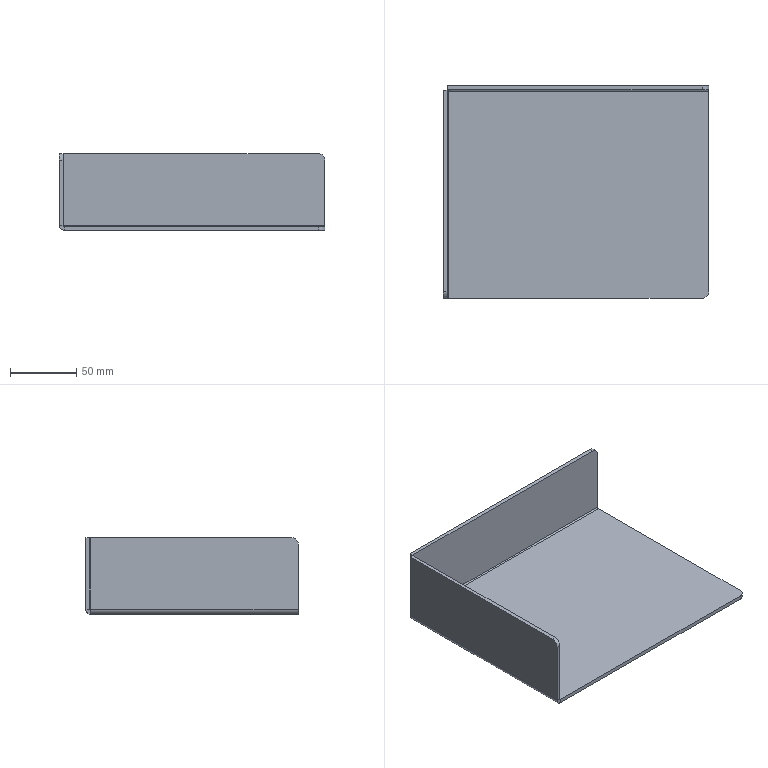Part | SolidWorks | features EdgeFlange 1, Fillet 1, FlatPattern 1, SMBaseFlange 1, SheetMetal 1 | 1 solid | 25 faces | box 200 x 160 x 58 mm | volume 153068 mm3 | plane 16 | cylinder 7 | spline 2 | commonest cylinder face diameters 10 x3 2 x2 8 x2
STEP:
#1=CARTESIAN_POINT('',(0.,5.,-3.));
#2=VERTEX_POINT('',#1);
#3=CARTESIAN_POINT('',(0.,156.,-3.));
#4=VERTEX_POINT('',#3);
#5=CARTESIAN_POINT('',(0.,0.,-3.));
#6=DIRECTION('',(0.,1.,0.));
#7=VECTOR('',#6,1000.);
#8=LINE('',#5,#7);
#9=EDGE_CURVE('',#2,#4,#8,.T.);
#10=ORIENTED_EDGE('',*,*,#9,.F.);
#11=CARTESIAN_POINT('',(-5.,0.,-3.));
#12=VERTEX_POINT('',#11);
#13=CARTESIAN_POINT('',(-5.,5.,-3.));
#14=DIRECTION('',(0.,0.,-1.));
#15=DIRECTION('',(1.,0.,0.));
#16=AXIS2_PLACEMENT_3D('',#13,#14,#15);
#17=CIRCLE('',#16,5.);
#18=EDGE_CURVE('',#2,#12,#17,.T.);
#19=ORIENTED_EDGE('',*,*,#18,.T.);
#20=CARTESIAN_POINT('',(-196.,0.,-3.));
#21=VERTEX_POINT('',#20);
#22=CARTESIAN_POINT('',(0.,0.,-3.));
#23=DIRECTION('',(1.,0.,0.));
#24=VECTOR('',#23,1000.);
#25=LINE('',#22,#24);
#26=EDGE_CURVE('',#21,#12,#25,.T.);
#27=ORIENTED_EDGE('',*,*,#26,.F.);
#28=CARTESIAN_POINT('',(-196.,156.,-3.));
#29=VERTEX_POINT('',#28);
#30=CARTESIAN_POINT('',(-196.,0.,-3.));
#31=DIRECTION('',(0.,1.,0.));
#32=VECTOR('',#31,1000.);
#33=LINE('',#30,#32);
#34=EDGE_CURVE('',#21,#29,#33,.T.);
#35=ORIENTED_EDGE('',*,*,#34,.T.);
#36=CARTESIAN_POINT('',(-196.646,156.,-3.));
#37=DIRECTION('',(1.,0.,0.));
#38=VECTOR('',#37,1000.);
#39=LINE('',#36,#38);
#40=EDGE_CURVE('',#29,#4,#39,.T.);
#41=ORIENTED_EDGE('',*,*,#40,.T.);
#42=EDGE_LOOP('',(#10,#19,#27,#35,#41));
#43=FACE_OUTER_BOUND('',#42,.T.);
#44=CARTESIAN_POINT('',(0.,0.,-3.));
#45=DIRECTION('',(0.,0.,1.));
#46=DIRECTION('',(1.,0.,0.));
#47=AXIS2_PLACEMENT_3D('',#44,#45,#46);
#48=PLANE('',#47);
#49=ADVANCED_FACE('',(#43),#48,.F.);
#50=CARTESIAN_POINT('',(-196.,0.,0.));
#51=VERTEX_POINT('',#50);
#52=CARTESIAN_POINT('',(-5.,0.,0.));
#53=VERTEX_POINT('',#52);
#54=CARTESIAN_POINT('',(0.,0.,0.));
#55=DIRECTION('',(1.,0.,0.));
#56=VECTOR('',#55,1000.);
#57=LINE('',#54,#56);
#58=EDGE_CURVE('',#51,#53,#57,.T.);
#59=ORIENTED_EDGE('',*,*,#58,.T.);
#60=CARTESIAN_POINT('',(0.,5.,0.));
#61=VERTEX_POINT('',#60);
#62=CARTESIAN_POINT('',(-5.,5.,0.));
#63=DIRECTION('',(0.,0.,1.));
#64=DIRECTION('',(1.,0.,0.));
#65=AXIS2_PLACEMENT_3D('',#62,#63,#64);
#66=CIRCLE('',#65,5.);
#67=EDGE_CURVE('',#53,#61,#66,.T.);
#68=ORIENTED_EDGE('',*,*,#67,.T.);
#69=CARTESIAN_POINT('',(0.,156.,0.));
#70=VERTEX_POINT('',#69);
#71=CARTESIAN_POINT('',(0.,0.,0.));
#72=DIRECTION('',(0.,1.,0.));
#73=VECTOR('',#72,1000.);
#74=LINE('',#71,#73);
#75=EDGE_CURVE('',#61,#70,#74,.T.);
#76=ORIENTED_EDGE('',*,*,#75,.T.);
#77=CARTESIAN_POINT('',(-196.,156.,0.));
#78=VERTEX_POINT('',#77);
#79=CARTESIAN_POINT('',(-196.646,156.,0.));
#80=DIRECTION('',(1.,0.,0.));
#81=VECTOR('',#80,1000.);
#82=LINE('',#79,#81);
#83=EDGE_CURVE('',#78,#70,#82,.T.);
#84=ORIENTED_EDGE('',*,*,#83,.F.);
#85=CARTESIAN_POINT('',(-196.,0.,0.));
#86=DIRECTION('',(0.,1.,0.));
#87=VECTOR('',#86,1000.);
#88=LINE('',#85,#87);
#89=EDGE_CURVE('',#51,#78,#88,.T.);
#90=ORIENTED_EDGE('',*,*,#89,.F.);
#91=EDGE_LOOP('',(#59,#68,#76,#84,#90));
#92=FACE_OUTER_BOUND('',#91,.T.);
#93=CARTESIAN_POINT('',(0.,0.,0.));
#94=DIRECTION('',(0.,0.,1.));
#95=DIRECTION('',(1.,0.,0.));
#96=AXIS2_PLACEMENT_3D('',#93,#94,#95);
#97=PLANE('',#96);
#98=ADVANCED_FACE('',(#92),#97,.T.);
#99=ORIENTED_EDGE('',*,*,#26,.T.);
#100=CARTESIAN_POINT('',(-5.,0.,-3.));
#101=DIRECTION('',(0.,0.,1.));
#102=VECTOR('',#101,1000.);
#103=LINE('',#100,#102);
#104=EDGE_CURVE('',#12,#53,#103,.T.);
#105=ORIENTED_EDGE('',*,*,#104,.T.);
#106=ORIENTED_EDGE('',*,*,#58,.F.);
#107=CARTESIAN_POINT('',(-196.,0.,0.));
#108=DIRECTION('',(0.,0.,-1.));
#109=VECTOR('',#108,1000.);
#110=LINE('',#107,#109);
#111=EDGE_CURVE('',#51,#21,#110,.T.);
#112=ORIENTED_EDGE('',*,*,#111,.T.);
#113=EDGE_LOOP('',(#99,#105,#106,#112));
#114=FACE_OUTER_BOUND('',#113,.T.);
#115=CARTESIAN_POINT('',(0.,0.,-3.));
#116=DIRECTION('',(0.,-1.,0.));
#117=DIRECTION('',(0.,0.,-1.));
#118=AXIS2_PLACEMENT_3D('',#115,#116,#117);
#119=PLANE('',#118);
#120=ADVANCED_FACE('',(#114),#119,.T.);
#121=ORIENTED_EDGE('',*,*,#75,.F.);
#122=CARTESIAN_POINT('',(0.,5.,-3.));
#123=DIRECTION('',(0.,0.,-1.));
#124=VECTOR('',#123,1000.);
#125=LINE('',#122,#124);
#126=EDGE_CURVE('',#61,#2,#125,.T.);
#127=ORIENTED_EDGE('',*,*,#126,.T.);
#128=ORIENTED_EDGE('',*,*,#9,.T.);
#129=CARTESIAN_POINT('',(0.,156.,0.));
#130=DIRECTION('',(0.,0.,-1.));
#131=VECTOR('',#130,1000.);
#132=LINE('',#129,#131);
#133=EDGE_CURVE('',#70,#4,#132,.T.);
#134=ORIENTED_EDGE('',*,*,#133,.F.);
#135=EDGE_LOOP('',(#121,#127,#128,#134));
#136=FACE_OUTER_BOUND('',#135,.T.);
#137=CARTESIAN_POINT('',(0.,0.,-3.));
#138=DIRECTION('',(1.,0.,0.));
#139=DIRECTION('',(0.,0.,-1.));
#140=AXIS2_PLACEMENT_3D('',#137,#138,#139);
#141=PLANE('',#140);
#142=ADVANCED_FACE('',(#136),#141,.T.);
#143=CARTESIAN_POINT('',(0.,157.,1.));
#144=VERTEX_POINT('',#143);
#145=CARTESIAN_POINT('',(0.,160.,1.));
#146=VERTEX_POINT('',#145);
#147=CARTESIAN_POINT('',(0.,160.,1.));
#148=DIRECTION('',(0.,1.,0.));
#149=VECTOR('',#148,1000.);
#150=LINE('',#147,#149);
#151=EDGE_CURVE('',#144,#146,#150,.T.);
#152=ORIENTED_EDGE('',*,*,#151,.F.);
#153=CARTESIAN_POINT('',(0.,156.,1.));
#154=DIRECTION('',(1.,0.,0.));
#155=DIRECTION('',(0.,0.,1.));
#156=AXIS2_PLACEMENT_3D('',#153,#154,#155);
#157=CIRCLE('',#156,1.);
#158=EDGE_CURVE('',#70,#144,#157,.T.);
#159=ORIENTED_EDGE('',*,*,#158,.F.);
#160=ORIENTED_EDGE('',*,*,#133,.T.);
#161=CARTESIAN_POINT('',(0.,156.,1.));
#162=DIRECTION('',(1.,0.,0.));
#163=DIRECTION('',(0.,0.,1.));
#164=AXIS2_PLACEMENT_3D('',#161,#162,#163);
#165=CIRCLE('',#164,4.);
#166=EDGE_CURVE('',#4,#146,#165,.T.);
#167=ORIENTED_EDGE('',*,*,#166,.T.);
#168=EDGE_LOOP('',(#152,#159,#160,#167));
#169=FACE_OUTER_BOUND('',#168,.T.);
#170=CARTESIAN_POINT('',(0.,156.,1.));
#171=DIRECTION('',(1.,0.,0.));
#172=DIRECTION('',(0.,0.,-1.));
#173=AXIS2_PLACEMENT_3D('',#170,#171,#172);
#174=PLANE('',#173);
#175=ADVANCED_FACE('',(#169),#174,.T.);
#176=CARTESIAN_POINT('',(-196.646,157.,1.));
#177=VERTEX_POINT('',#176);
#178=CARTESIAN_POINT('',(-196.646,157.,1.));
#179=CARTESIAN_POINT('',(-196.592,157.,0.8679));
#180=CARTESIAN_POINT('',(-196.539,156.974,0.7389));
#181=CARTESIAN_POINT('',(-196.431,156.874,0.4958));
#182=CARTESIAN_POINT('',(-196.377,156.8,0.3857));
#183=CARTESIAN_POINT('',(-196.215,156.522,0.1076));
#184=CARTESIAN_POINT('',(-196.109,156.264,0.));
#185=CARTESIAN_POINT('',(-196.,156.,0.));
#186=B_SPLINE_CURVE_WITH_KNOTS('',3,(#178,#179,#180,#181,#182,#183,#184,#185),.UNSPECIFIED.,.F.,.F.,(4,2,2,4),(0.,0.0004224,0.0008448,0.00169),.UNSPECIFIED.);
#187=EDGE_CURVE('',#177,#78,#186,.T.);
#188=ORIENTED_EDGE('',*,*,#187,.F.);
#189=CARTESIAN_POINT('',(-196.646,160.,1.));
#190=VERTEX_POINT('',#189);
#191=CARTESIAN_POINT('',(-196.646,157.,1.));
#192=DIRECTION('',(0.,-1.,0.));
#193=VECTOR('',#192,1000.);
#194=LINE('',#191,#193);
#195=EDGE_CURVE('',#190,#177,#194,.T.);
#196=ORIENTED_EDGE('',*,*,#195,.F.);
#197=CARTESIAN_POINT('',(-196.646,160.,1.));
#198=CARTESIAN_POINT('',(-196.592,160.,0.4714));
#199=CARTESIAN_POINT('',(-196.54,159.899,-0.03873));
#200=CARTESIAN_POINT('',(-196.458,159.596,-0.7708));
#201=CARTESIAN_POINT('',(-196.431,159.473,-1.001));
#202=CARTESIAN_POINT('',(-196.378,159.184,-1.435));
#203=CARTESIAN_POINT('',(-196.351,159.016,-1.641));
#204=CARTESIAN_POINT('',(-196.297,158.646,-2.012));
#205=CARTESIAN_POINT('',(-196.27,158.444,-2.177));
#206=CARTESIAN_POINT('',(-196.216,158.01,-2.468));
#207=CARTESIAN_POINT('',(-196.189,157.775,-2.594));
#208=CARTESIAN_POINT('',(-196.135,157.293,-2.794));
#209=CARTESIAN_POINT('',(-196.108,157.044,-2.87));
#210=CARTESIAN_POINT('',(-196.054,156.528,-2.974));
#211=CARTESIAN_POINT('',(-196.027,156.264,-3.));
#212=CARTESIAN_POINT('',(-196.,156.,-3.));
#213=B_SPLINE_CURVE_WITH_KNOTS('',3,(#197,#198,#199,#200,#201,#202,#203,#204,#205,#206,#207,#208,#209,#210,#211,#212),.UNSPECIFIED.,.F.,.F.,(4,2,2,2,2,2,2,4),(0.,0.001565,0.002347,0.00313,0.003912,0.004695,0.005477,0.00626),.UNSPECIFIED.);
#214=EDGE_CURVE('',#190,#29,#213,.T.);
#215=ORIENTED_EDGE('',*,*,#214,.T.);
#216=CARTESIAN_POINT('',(-196.,156.,0.));
#217=DIRECTION('',(0.,0.,-1.));
#218=VECTOR('',#217,1000.);
#219=LINE('',#216,#218);
#220=EDGE_CURVE('',#78,#29,#219,.T.);
#221=ORIENTED_EDGE('',*,*,#220,.F.);
#222=EDGE_LOOP('',(#188,#196,#215,#221));
#223=FACE_OUTER_BOUND('',#222,.T.);
#224=CARTESIAN_POINT('',(-196.646,160.03,1.));
#225=CARTESIAN_POINT('',(-196.593,160.03,0.4724));
#226=CARTESIAN_POINT('',(-196.539,159.925,-0.05484));
#227=CARTESIAN_POINT('',(-196.431,159.521,-1.03));
#228=CARTESIAN_POINT('',(-196.377,159.223,-1.477));
#229=CARTESIAN_POINT('',(-196.269,158.477,-2.223));
#230=CARTESIAN_POINT('',(-196.215,158.03,-2.521));
#231=CARTESIAN_POINT('',(-196.108,157.055,-2.925));
#232=CARTESIAN_POINT('',(-196.054,156.528,-3.03));
#233=CARTESIAN_POINT('',(-196.,156.,-3.03));
#234=CARTESIAN_POINT('',(-196.646,160.,1.));
#235=CARTESIAN_POINT('',(-196.593,160.,0.4763));
#236=CARTESIAN_POINT('',(-196.539,159.896,-0.04699));
#237=CARTESIAN_POINT('',(-196.431,159.495,-1.014));
#238=CARTESIAN_POINT('',(-196.377,159.199,-1.458));
#239=CARTESIAN_POINT('',(-196.269,158.458,-2.199));
#240=CARTESIAN_POINT('',(-196.215,158.014,-2.495));
#241=CARTESIAN_POINT('',(-196.108,157.047,-2.896));
#242=CARTESIAN_POINT('',(-196.054,156.524,-3.));
#243=CARTESIAN_POINT('',(-196.,156.,-3.));
#244=CARTESIAN_POINT('',(-196.646,157.,1.));
#245=CARTESIAN_POINT('',(-196.593,157.,0.8691));
#246=CARTESIAN_POINT('',(-196.539,156.974,0.7383));
#247=CARTESIAN_POINT('',(-196.431,156.874,0.4964));
#248=CARTESIAN_POINT('',(-196.377,156.8,0.3855));
#249=CARTESIAN_POINT('',(-196.269,156.615,0.2003));
#250=CARTESIAN_POINT('',(-196.215,156.504,0.1262));
#251=CARTESIAN_POINT('',(-196.108,156.262,0.02603));
#252=CARTESIAN_POINT('',(-196.054,156.131,0.));
#253=CARTESIAN_POINT('',(-196.,156.,0.));
#254=CARTESIAN_POINT('',(-196.646,156.97,1.));
#255=CARTESIAN_POINT('',(-196.593,156.97,0.873));
#256=CARTESIAN_POINT('',(-196.539,156.944,0.7462));
#257=CARTESIAN_POINT('',(-196.431,156.847,0.5116));
#258=CARTESIAN_POINT('',(-196.377,156.775,0.4041));
#259=CARTESIAN_POINT('',(-196.269,156.596,0.2246));
#260=CARTESIAN_POINT('',(-196.215,156.488,0.1527));
#261=CARTESIAN_POINT('',(-196.108,156.254,0.05554));
#262=CARTESIAN_POINT('',(-196.054,156.127,0.0303));
#263=CARTESIAN_POINT('',(-196.,156.,0.0303));
#264=B_SPLINE_SURFACE_WITH_KNOTS('',1,3,((#224,#225,#226,#227,#228,#229,#230,#231,#232,#233),(#234,#235,#236,#237,#238,#239,#240,#241,#242,#243),(#244,#245,#246,#247,#248,#249,#250,#251,#252,#253),(#254,#255,#256,#257,#258,#259,#260,#261,#262,#263)),.UNSPECIFIED.,.F.,.F.,.F.,(2,1,1,2),(4,2,2,2,4),(-0.01,0.,1.,1.01),(0.,0.25,0.5,0.75,1.),.UNSPECIFIED.);
#265=ADVANCED_FACE('',(#223),#264,.F.);
#266=ORIENTED_EDGE('',*,*,#40,.F.);
#267=ORIENTED_EDGE('',*,*,#214,.F.);
#268=CARTESIAN_POINT('',(0.,160.,1.));
#269=DIRECTION('',(1.,0.,0.));
#270=VECTOR('',#269,1000.);
#271=LINE('',#268,#270);
#272=EDGE_CURVE('',#190,#146,#271,.T.);
#273=ORIENTED_EDGE('',*,*,#272,.T.);
#274=ORIENTED_EDGE('',*,*,#166,.F.);
#275=EDGE_LOOP('',(#266,#267,#273,#274));
#276=FACE_OUTER_BOUND('',#275,.T.);
#277=CARTESIAN_POINT('',(-196.646,156.,1.));
#278=DIRECTION('',(-1.,0.,0.));
#279=DIRECTION('',(0.,1.,0.));
#280=AXIS2_PLACEMENT_3D('',#277,#278,#279);
#281=CYLINDRICAL_SURFACE('',#280,4.);
#282=ADVANCED_FACE('',(#276),#281,.T.);
#283=ORIENTED_EDGE('',*,*,#83,.T.);
#284=ORIENTED_EDGE('',*,*,#158,.T.);
#285=CARTESIAN_POINT('',(0.,157.,1.));
#286=DIRECTION('',(-1.,0.,0.));
#287=VECTOR('',#286,1000.);
#288=LINE('',#285,#287);
#289=EDGE_CURVE('',#144,#177,#288,.T.);
#290=ORIENTED_EDGE('',*,*,#289,.T.);
#291=ORIENTED_EDGE('',*,*,#187,.T.);
#292=EDGE_LOOP('',(#283,#284,#290,#291));
#293=FACE_OUTER_BOUND('',#292,.T.);
#294=CARTESIAN_POINT('',(-196.646,156.,1.));
#295=DIRECTION('',(-1.,0.,0.));
#296=DIRECTION('',(0.,1.,0.));
#297=AXIS2_PLACEMENT_3D('',#294,#295,#296);
#298=CYLINDRICAL_SURFACE('',#297,1.);
#299=ADVANCED_FACE('',(#293),#298,.F.);
#300=CARTESIAN_POINT('',(0.,160.,50.));
#301=VERTEX_POINT('',#300);
#302=CARTESIAN_POINT('',(0.,160.,0.));
#303=DIRECTION('',(0.,0.,-1.));
#304=VECTOR('',#303,1000.);
#305=LINE('',#302,#304);
#306=EDGE_CURVE('',#301,#146,#305,.T.);
#307=ORIENTED_EDGE('',*,*,#306,.F.);
#308=CARTESIAN_POINT('',(0.,157.,50.));
#309=VERTEX_POINT('',#308);
#310=CARTESIAN_POINT('',(0.,160.,50.));
#311=DIRECTION('',(0.,-1.,0.));
#312=VECTOR('',#311,1000.);
#313=LINE('',#310,#312);
#314=EDGE_CURVE('',#301,#309,#313,.T.);
#315=ORIENTED_EDGE('',*,*,#314,.T.);
#316=CARTESIAN_POINT('',(0.,157.,0.));
#317=DIRECTION('',(0.,0.,-1.));
#318=VECTOR('',#317,1000.);
#319=LINE('',#316,#318);
#320=EDGE_CURVE('',#309,#144,#319,.T.);
#321=ORIENTED_EDGE('',*,*,#320,.T.);
#322=ORIENTED_EDGE('',*,*,#151,.T.);
#323=EDGE_LOOP('',(#307,#315,#321,#322));
#324=FACE_OUTER_BOUND('',#323,.T.);
#325=CARTESIAN_POINT('',(0.,160.,0.));
#326=DIRECTION('',(-1.,0.,0.));
#327=DIRECTION('',(0.,-1.,0.));
#328=AXIS2_PLACEMENT_3D('',#325,#326,#327);
#329=PLANE('',#328);
#330=ADVANCED_FACE('',(#324),#329,.F.);
#331=CARTESIAN_POINT('',(-196.646,160.,55.));
#332=VERTEX_POINT('',#331);
#333=CARTESIAN_POINT('',(-5.,160.,55.));
#334=VERTEX_POINT('',#333);
#335=CARTESIAN_POINT('',(0.,160.,55.));
#336=DIRECTION('',(1.,0.,0.));
#337=VECTOR('',#336,1000.);
#338=LINE('',#335,#337);
#339=EDGE_CURVE('',#332,#334,#338,.T.);
#340=ORIENTED_EDGE('',*,*,#339,.T.);
#341=CARTESIAN_POINT('',(-5.,160.,50.));
#342=DIRECTION('',(0.,1.,0.));
#343=DIRECTION('',(0.,0.,-1.));
#344=AXIS2_PLACEMENT_3D('',#341,#342,#343);
#345=CIRCLE('',#344,5.);
#346=EDGE_CURVE('',#334,#301,#345,.T.);
#347=ORIENTED_EDGE('',*,*,#346,.T.);
#348=ORIENTED_EDGE('',*,*,#306,.T.);
#349=ORIENTED_EDGE('',*,*,#272,.F.);
#350=CARTESIAN_POINT('',(-196.646,160.,0.));
#351=DIRECTION('',(0.,0.,1.));
#352=VECTOR('',#351,1000.);
#353=LINE('',#350,#352);
#354=EDGE_CURVE('',#190,#332,#353,.T.);
#355=ORIENTED_EDGE('',*,*,#354,.T.);
#356=EDGE_LOOP('',(#340,#347,#348,#349,#355));
#357=FACE_OUTER_BOUND('',#356,.T.);
#358=CARTESIAN_POINT('',(0.,160.,0.));
#359=DIRECTION('',(0.,-1.,0.));
#360=DIRECTION('',(0.,0.,-1.));
#361=AXIS2_PLACEMENT_3D('',#358,#359,#360);
#362=PLANE('',#361);
#363=ADVANCED_FACE('',(#357),#362,.F.);
#364=ORIENTED_EDGE('',*,*,#320,.F.);
#365=CARTESIAN_POINT('',(-5.,157.,55.));
#366=VERTEX_POINT('',#365);
#367=CARTESIAN_POINT('',(-5.,157.,50.));
#368=DIRECTION('',(0.,-1.,0.));
#369=DIRECTION('',(0.,0.,-1.));
#370=AXIS2_PLACEMENT_3D('',#367,#368,#369);
#371=CIRCLE('',#370,5.);
#372=EDGE_CURVE('',#309,#366,#371,.T.);
#373=ORIENTED_EDGE('',*,*,#372,.T.);
#374=CARTESIAN_POINT('',(-196.646,157.,55.));
#375=VERTEX_POINT('',#374);
#376=CARTESIAN_POINT('',(0.,157.,55.));
#377=DIRECTION('',(1.,0.,0.));
#378=VECTOR('',#377,1000.);
#379=LINE('',#376,#378);
#380=EDGE_CURVE('',#375,#366,#379,.T.);
#381=ORIENTED_EDGE('',*,*,#380,.F.);
#382=CARTESIAN_POINT('',(-196.646,157.,0.));
#383=DIRECTION('',(0.,0.,1.));
#384=VECTOR('',#383,1000.);
#385=LINE('',#382,#384);
#386=EDGE_CURVE('',#177,#375,#385,.T.);
#387=ORIENTED_EDGE('',*,*,#386,.F.);
#388=ORIENTED_EDGE('',*,*,#289,.F.);
#389=EDGE_LOOP('',(#364,#373,#381,#387,#388));
#390=FACE_OUTER_BOUND('',#389,.T.);
#391=CARTESIAN_POINT('',(0.,157.,0.));
#392=DIRECTION('',(0.,-1.,0.));
#393=DIRECTION('',(0.,0.,-1.));
#394=AXIS2_PLACEMENT_3D('',#391,#392,#393);
#395=PLANE('',#394);
#396=ADVANCED_FACE('',(#390),#395,.T.);
#397=ORIENTED_EDGE('',*,*,#380,.T.);
#398=CARTESIAN_POINT('',(-5.,160.,55.));
#399=DIRECTION('',(0.,1.,0.));
#400=VECTOR('',#399,1000.);
#401=LINE('',#398,#400);
#402=EDGE_CURVE('',#366,#334,#401,.T.);
#403=ORIENTED_EDGE('',*,*,#402,.T.);
#404=ORIENTED_EDGE('',*,*,#339,.F.);
#405=CARTESIAN_POINT('',(-196.646,160.,55.));
#406=DIRECTION('',(0.,-1.,0.));
#407=VECTOR('',#406,1000.);
#408=LINE('',#405,#407);
#409=EDGE_CURVE('',#332,#375,#408,.T.);
#410=ORIENTED_EDGE('',*,*,#409,.T.);
#411=EDGE_LOOP('',(#397,#403,#404,#410));
#412=FACE_OUTER_BOUND('',#411,.T.);
#413=CARTESIAN_POINT('',(0.,160.,55.));
#414=DIRECTION('',(0.,0.,-1.));
#415=DIRECTION('',(0.,1.,0.));
#416=AXIS2_PLACEMENT_3D('',#413,#414,#415);
#417=PLANE('',#416);
#418=ADVANCED_FACE('',(#412),#417,.F.);
#419=ORIENTED_EDGE('',*,*,#409,.F.);
#420=ORIENTED_EDGE('',*,*,#354,.F.);
#421=ORIENTED_EDGE('',*,*,#195,.T.);
#422=ORIENTED_EDGE('',*,*,#386,.T.);
#423=EDGE_LOOP('',(#419,#420,#421,#422));
#424=FACE_OUTER_BOUND('',#423,.T.);
#425=CARTESIAN_POINT('',(-196.646,157.,0.));
#426=DIRECTION('',(1.,0.,0.));
#427=DIRECTION('',(0.,0.,-1.));
#428=AXIS2_PLACEMENT_3D('',#425,#426,#427);
#429=PLANE('',#428);
#430=ADVANCED_FACE('',(#424),#429,.F.);
#431=CARTESIAN_POINT('',(-200.,156.646,1.));
#432=VERTEX_POINT('',#431);
#433=CARTESIAN_POINT('',(-197.,156.646,1.));
#434=VERTEX_POINT('',#433);
#435=CARTESIAN_POINT('',(-197.,156.646,1.));
#436=DIRECTION('',(1.,0.,0.));
#437=VECTOR('',#436,1000.);
#438=LINE('',#435,#437);
#439=EDGE_CURVE('',#432,#434,#438,.T.);
#440=ORIENTED_EDGE('',*,*,#439,.T.);
#441=CARTESIAN_POINT('',(-196.,156.,0.));
#442=CARTESIAN_POINT('',(-196.132,156.054,0.));
#443=CARTESIAN_POINT('',(-196.261,156.107,0.02577));
#444=CARTESIAN_POINT('',(-196.504,156.216,0.1264));
#445=CARTESIAN_POINT('',(-196.614,156.269,0.2001));
#446=CARTESIAN_POINT('',(-196.892,156.431,0.4782));
#447=CARTESIAN_POINT('',(-197.,156.538,0.7358));
#448=CARTESIAN_POINT('',(-197.,156.646,1.));
#449=B_SPLINE_CURVE_WITH_KNOTS('',3,(#441,#442,#443,#444,#445,#446,#447,#448),.UNSPECIFIED.,.F.,.F.,(4,2,2,4),(0.,0.0004224,0.0008448,0.00169),.UNSPECIFIED.);
#450=EDGE_CURVE('',#78,#434,#449,.T.);
#451=ORIENTED_EDGE('',*,*,#450,.F.);
#452=ORIENTED_EDGE('',*,*,#220,.T.);
#453=CARTESIAN_POINT('',(-196.,156.,-3.));
#454=CARTESIAN_POINT('',(-196.529,156.054,-3.));
#455=CARTESIAN_POINT('',(-197.039,156.107,-2.899));
#456=CARTESIAN_POINT('',(-197.771,156.188,-2.596));
#457=CARTESIAN_POINT('',(-198.001,156.215,-2.473));
#458=CARTESIAN_POINT('',(-198.435,156.269,-2.184));
#459=CARTESIAN_POINT('',(-198.641,156.296,-2.016));
#460=CARTESIAN_POINT('',(-199.012,156.35,-1.646));
#461=CARTESIAN_POINT('',(-199.177,156.377,-1.444));
#462=CARTESIAN_POINT('',(-199.468,156.43,-1.01));
#463=CARTESIAN_POINT('',(-199.594,156.458,-0.7752));
#464=CARTESIAN_POINT('',(-199.794,156.511,-0.2932));
#465=CARTESIAN_POINT('',(-199.87,156.538,-0.04382));
#466=CARTESIAN_POINT('',(-199.974,156.592,0.4721));
#467=CARTESIAN_POINT('',(-200.,156.619,0.7357));
#468=CARTESIAN_POINT('',(-200.,156.646,1.));
#469=B_SPLINE_CURVE_WITH_KNOTS('',3,(#453,#454,#455,#456,#457,#458,#459,#460,#461,#462,#463,#464,#465,#466,#467,#468),.UNSPECIFIED.,.F.,.F.,(4,2,2,2,2,2,2,4),(0.,0.001565,0.002347,0.00313,0.003912,0.004695,0.005477,0.00626),.UNSPECIFIED.);
#470=EDGE_CURVE('',#29,#432,#469,.T.);
#471=ORIENTED_EDGE('',*,*,#470,.T.);
#472=EDGE_LOOP('',(#440,#451,#452,#471));
#473=FACE_OUTER_BOUND('',#472,.T.);
#474=CARTESIAN_POINT('',(-196.,156.,-3.03));
#475=CARTESIAN_POINT('',(-196.528,156.054,-3.03));
#476=CARTESIAN_POINT('',(-197.055,156.108,-2.925));
#477=CARTESIAN_POINT('',(-198.03,156.215,-2.521));
#478=CARTESIAN_POINT('',(-198.477,156.269,-2.223));
#479=CARTESIAN_POINT('',(-199.223,156.377,-1.477));
#480=CARTESIAN_POINT('',(-199.521,156.431,-1.03));
#481=CARTESIAN_POINT('',(-199.925,156.539,-0.05484));
#482=CARTESIAN_POINT('',(-200.03,156.593,0.4724));
#483=CARTESIAN_POINT('',(-200.03,156.646,1.));
#484=CARTESIAN_POINT('',(-196.,156.,-3.));
#485=CARTESIAN_POINT('',(-196.524,156.054,-3.));
#486=CARTESIAN_POINT('',(-197.047,156.108,-2.896));
#487=CARTESIAN_POINT('',(-198.014,156.215,-2.495));
#488=CARTESIAN_POINT('',(-198.458,156.269,-2.199));
#489=CARTESIAN_POINT('',(-199.199,156.377,-1.458));
#490=CARTESIAN_POINT('',(-199.495,156.431,-1.014));
#491=CARTESIAN_POINT('',(-199.896,156.539,-0.04699));
#492=CARTESIAN_POINT('',(-200.,156.593,0.4763));
#493=CARTESIAN_POINT('',(-200.,156.646,1.));
#494=CARTESIAN_POINT('',(-196.,156.,0.));
#495=CARTESIAN_POINT('',(-196.131,156.054,0.));
#496=CARTESIAN_POINT('',(-196.262,156.108,0.02603));
#497=CARTESIAN_POINT('',(-196.504,156.215,0.1262));
#498=CARTESIAN_POINT('',(-196.615,156.269,0.2003));
#499=CARTESIAN_POINT('',(-196.8,156.377,0.3855));
#500=CARTESIAN_POINT('',(-196.874,156.431,0.4964));
#501=CARTESIAN_POINT('',(-196.974,156.539,0.7383));
#502=CARTESIAN_POINT('',(-197.,156.593,0.8691));
#503=CARTESIAN_POINT('',(-197.,156.646,1.));
#504=CARTESIAN_POINT('',(-196.,156.,0.0303));
#505=CARTESIAN_POINT('',(-196.127,156.054,0.0303));
#506=CARTESIAN_POINT('',(-196.254,156.108,0.05554));
#507=CARTESIAN_POINT('',(-196.488,156.215,0.1527));
#508=CARTESIAN_POINT('',(-196.596,156.269,0.2246));
#509=CARTESIAN_POINT('',(-196.775,156.377,0.4041));
#510=CARTESIAN_POINT('',(-196.847,156.431,0.5116));
#511=CARTESIAN_POINT('',(-196.944,156.539,0.7462));
#512=CARTESIAN_POINT('',(-196.97,156.593,0.873));
#513=CARTESIAN_POINT('',(-196.97,156.646,1.));
#514=B_SPLINE_SURFACE_WITH_KNOTS('',1,3,((#474,#475,#476,#477,#478,#479,#480,#481,#482,#483),(#484,#485,#486,#487,#488,#489,#490,#491,#492,#493),(#494,#495,#496,#497,#498,#499,#500,#501,#502,#503),(#504,#505,#506,#507,#508,#509,#510,#511,#512,#513)),.UNSPECIFIED.,.F.,.F.,.F.,(2,1,1,2),(4,2,2,2,4),(-0.01,0.,1.,1.01),(0.,0.25,0.5,0.75,1.),.UNSPECIFIED.);
#515=ADVANCED_FACE('',(#473),#514,.F.);
#516=CARTESIAN_POINT('',(-197.,0.,1.));
#517=VERTEX_POINT('',#516);
#518=CARTESIAN_POINT('',(-196.,0.,1.));
#519=DIRECTION('',(0.,-1.,0.));
#520=DIRECTION('',(0.,0.,-1.));
#521=AXIS2_PLACEMENT_3D('',#518,#519,#520);
#522=CIRCLE('',#521,1.);
#523=EDGE_CURVE('',#517,#51,#522,.T.);
#524=ORIENTED_EDGE('',*,*,#523,.F.);
#525=CARTESIAN_POINT('',(-200.,0.,1.));
#526=VERTEX_POINT('',#525);
#527=CARTESIAN_POINT('',(-197.,0.,1.));
#528=DIRECTION('',(-1.,0.,0.));
#529=VECTOR('',#528,1000.);
#530=LINE('',#527,#529);
#531=EDGE_CURVE('',#517,#526,#530,.T.);
#532=ORIENTED_EDGE('',*,*,#531,.T.);
#533=CARTESIAN_POINT('',(-196.,0.,1.));
#534=DIRECTION('',(0.,-1.,0.));
#535=DIRECTION('',(0.,0.,-1.));
#536=AXIS2_PLACEMENT_3D('',#533,#534,#535);
#537=CIRCLE('',#536,4.);
#538=EDGE_CURVE('',#526,#21,#537,.T.);
#539=ORIENTED_EDGE('',*,*,#538,.T.);
#540=ORIENTED_EDGE('',*,*,#111,.F.);
#541=EDGE_LOOP('',(#524,#532,#539,#540));
#542=FACE_OUTER_BOUND('',#541,.T.);
#543=CARTESIAN_POINT('',(-196.,0.,1.));
#544=DIRECTION('',(0.,1.,0.));
#545=DIRECTION('',(0.,0.,1.));
#546=AXIS2_PLACEMENT_3D('',#543,#544,#545);
#547=PLANE('',#546);
#548=ADVANCED_FACE('',(#542),#547,.F.);
#549=ORIENTED_EDGE('',*,*,#34,.F.);
#550=ORIENTED_EDGE('',*,*,#538,.F.);
#551=CARTESIAN_POINT('',(-200.,160.,1.));
#552=DIRECTION('',(0.,1.,0.));
#553=VECTOR('',#552,1000.);
#554=LINE('',#551,#553);
#555=EDGE_CURVE('',#526,#432,#554,.T.);
#556=ORIENTED_EDGE('',*,*,#555,.T.);
#557=ORIENTED_EDGE('',*,*,#470,.F.);
#558=EDGE_LOOP('',(#549,#550,#556,#557));
#559=FACE_OUTER_BOUND('',#558,.T.);
#560=CARTESIAN_POINT('',(-196.,0.,1.));
#561=DIRECTION('',(0.,-1.,0.));
#562=DIRECTION('',(-1.,0.,0.));
#563=AXIS2_PLACEMENT_3D('',#560,#561,#562);
#564=CYLINDRICAL_SURFACE('',#563,4.);
#565=ADVANCED_FACE('',(#559),#564,.T.);
#566=ORIENTED_EDGE('',*,*,#89,.T.);
#567=ORIENTED_EDGE('',*,*,#450,.T.);
#568=CARTESIAN_POINT('',(-197.,160.,1.));
#569=DIRECTION('',(0.,-1.,0.));
#570=VECTOR('',#569,1000.);
#571=LINE('',#568,#570);
#572=EDGE_CURVE('',#434,#517,#571,.T.);
#573=ORIENTED_EDGE('',*,*,#572,.T.);
#574=ORIENTED_EDGE('',*,*,#523,.T.);
#575=EDGE_LOOP('',(#566,#567,#573,#574));
#576=FACE_OUTER_BOUND('',#575,.T.);
#577=CARTESIAN_POINT('',(-196.,0.,1.));
#578=DIRECTION('',(0.,-1.,0.));
#579=DIRECTION('',(-1.,0.,0.));
#580=AXIS2_PLACEMENT_3D('',#577,#578,#579);
#581=CYLINDRICAL_SURFACE('',#580,1.);
#582=ADVANCED_FACE('',(#576),#581,.F.);
#583=CARTESIAN_POINT('',(-200.,156.646,55.));
#584=VERTEX_POINT('',#583);
#585=CARTESIAN_POINT('',(-200.,156.646,0.));
#586=DIRECTION('',(0.,0.,1.));
#587=VECTOR('',#586,1000.);
#588=LINE('',#585,#587);
#589=EDGE_CURVE('',#432,#584,#588,.T.);
#590=ORIENTED_EDGE('',*,*,#589,.T.);
#591=CARTESIAN_POINT('',(-197.,156.646,55.));
#592=VERTEX_POINT('',#591);
#593=CARTESIAN_POINT('',(-197.,156.646,55.));
#594=DIRECTION('',(1.,0.,0.));
#595=VECTOR('',#594,1000.);
#596=LINE('',#593,#595);
#597=EDGE_CURVE('',#584,#592,#596,.T.);
#598=ORIENTED_EDGE('',*,*,#597,.T.);
#599=CARTESIAN_POINT('',(-197.,156.646,0.));
#600=DIRECTION('',(0.,0.,1.));
#601=VECTOR('',#600,1000.);
#602=LINE('',#599,#601);
#603=EDGE_CURVE('',#434,#592,#602,.T.);
#604=ORIENTED_EDGE('',*,*,#603,.F.);
#605=ORIENTED_EDGE('',*,*,#439,.F.);
#606=EDGE_LOOP('',(#590,#598,#604,#605));
#607=FACE_OUTER_BOUND('',#606,.T.);
#608=CARTESIAN_POINT('',(-197.,156.646,0.));
#609=DIRECTION('',(0.,1.,0.));
#610=DIRECTION('',(0.,0.,1.));
#611=AXIS2_PLACEMENT_3D('',#608,#609,#610);
#612=PLANE('',#611);
#613=ADVANCED_FACE('',(#607),#612,.T.);
#614=CARTESIAN_POINT('',(-200.,0.,50.));
#615=VERTEX_POINT('',#614);
#616=CARTESIAN_POINT('',(-200.,0.,0.));
#617=DIRECTION('',(0.,0.,1.));
#618=VECTOR('',#617,1000.);
#619=LINE('',#616,#618);
#620=EDGE_CURVE('',#526,#615,#619,.T.);
#621=ORIENTED_EDGE('',*,*,#620,.T.);
#622=CARTESIAN_POINT('',(-200.,5.,55.));
#623=VERTEX_POINT('',#622);
#624=CARTESIAN_POINT('',(-200.,5.,50.));
#625=DIRECTION('',(-1.,0.,0.));
#626=DIRECTION('',(0.,0.,-1.));
#627=AXIS2_PLACEMENT_3D('',#624,#625,#626);
#628=CIRCLE('',#627,5.);
#629=EDGE_CURVE('',#615,#623,#628,.T.);
#630=ORIENTED_EDGE('',*,*,#629,.T.);
#631=CARTESIAN_POINT('',(-200.,0.,55.));
#632=DIRECTION('',(0.,1.,0.));
#633=VECTOR('',#632,1000.);
#634=LINE('',#631,#633);
#635=EDGE_CURVE('',#623,#584,#634,.T.);
#636=ORIENTED_EDGE('',*,*,#635,.T.);
#637=ORIENTED_EDGE('',*,*,#589,.F.);
#638=ORIENTED_EDGE('',*,*,#555,.F.);
#639=EDGE_LOOP('',(#621,#630,#636,#637,#638));
#640=FACE_OUTER_BOUND('',#639,.T.);
#641=CARTESIAN_POINT('',(-200.,0.,0.));
#642=DIRECTION('',(1.,0.,0.));
#643=DIRECTION('',(0.,0.,-1.));
#644=AXIS2_PLACEMENT_3D('',#641,#642,#643);
#645=PLANE('',#644);
#646=ADVANCED_FACE('',(#640),#645,.F.);
#647=CARTESIAN_POINT('',(-197.,5.,55.));
#648=VERTEX_POINT('',#647);
#649=CARTESIAN_POINT('',(-197.,160.,55.));
#650=DIRECTION('',(0.,1.,0.));
#651=VECTOR('',#650,1000.);
#652=LINE('',#649,#651);
#653=EDGE_CURVE('',#648,#592,#652,.T.);
#654=ORIENTED_EDGE('',*,*,#653,.F.);
#655=CARTESIAN_POINT('',(-197.,0.,50.));
#656=VERTEX_POINT('',#655);
#657=CARTESIAN_POINT('',(-197.,5.,50.));
#658=DIRECTION('',(1.,0.,0.));
#659=DIRECTION('',(0.,0.,-1.));
#660=AXIS2_PLACEMENT_3D('',#657,#658,#659);
#661=CIRCLE('',#660,5.);
#662=EDGE_CURVE('',#648,#656,#661,.T.);
#663=ORIENTED_EDGE('',*,*,#662,.T.);
#664=CARTESIAN_POINT('',(-197.,0.,55.));
#665=DIRECTION('',(0.,0.,1.));
#666=VECTOR('',#665,1000.);
#667=LINE('',#664,#666);
#668=EDGE_CURVE('',#517,#656,#667,.T.);
#669=ORIENTED_EDGE('',*,*,#668,.F.);
#670=ORIENTED_EDGE('',*,*,#572,.F.);
#671=ORIENTED_EDGE('',*,*,#603,.T.);
#672=EDGE_LOOP('',(#654,#663,#669,#670,#671));
#673=FACE_OUTER_BOUND('',#672,.T.);
#674=CARTESIAN_POINT('',(-197.,0.,0.));
#675=DIRECTION('',(1.,0.,0.));
#676=DIRECTION('',(0.,0.,-1.));
#677=AXIS2_PLACEMENT_3D('',#674,#675,#676);
#678=PLANE('',#677);
#679=ADVANCED_FACE('',(#673),#678,.T.);
#680=ORIENTED_EDGE('',*,*,#635,.F.);
#681=CARTESIAN_POINT('',(-200.,5.,55.));
#682=DIRECTION('',(1.,0.,0.));
#683=VECTOR('',#682,1000.);
#684=LINE('',#681,#683);
#685=EDGE_CURVE('',#623,#648,#684,.T.);
#686=ORIENTED_EDGE('',*,*,#685,.T.);
#687=ORIENTED_EDGE('',*,*,#653,.T.);
#688=ORIENTED_EDGE('',*,*,#597,.F.);
#689=EDGE_LOOP('',(#680,#686,#687,#688));
#690=FACE_OUTER_BOUND('',#689,.T.);
#691=CARTESIAN_POINT('',(-200.,160.,55.));
#692=DIRECTION('',(0.,0.,-1.));
#693=DIRECTION('',(-1.,0.,0.));
#694=AXIS2_PLACEMENT_3D('',#691,#692,#693);
#695=PLANE('',#694);
#696=ADVANCED_FACE('',(#690),#695,.F.);
#697=ORIENTED_EDGE('',*,*,#668,.T.);
#698=CARTESIAN_POINT('',(-200.,0.,50.));
#699=DIRECTION('',(-1.,0.,0.));
#700=VECTOR('',#699,1000.);
#701=LINE('',#698,#700);
#702=EDGE_CURVE('',#656,#615,#701,.T.);
#703=ORIENTED_EDGE('',*,*,#702,.T.);
#704=ORIENTED_EDGE('',*,*,#620,.F.);
#705=ORIENTED_EDGE('',*,*,#531,.F.);
#706=EDGE_LOOP('',(#697,#703,#704,#705));
#707=FACE_OUTER_BOUND('',#706,.T.);
#708=CARTESIAN_POINT('',(-200.,0.,55.));
#709=DIRECTION('',(0.,1.,0.));
#710=DIRECTION('',(0.,0.,1.));
#711=AXIS2_PLACEMENT_3D('',#708,#709,#710);
#712=PLANE('',#711);
#713=ADVANCED_FACE('',(#707),#712,.F.);
#714=ORIENTED_EDGE('',*,*,#629,.F.);
#715=ORIENTED_EDGE('',*,*,#702,.F.);
#716=ORIENTED_EDGE('',*,*,#662,.F.);
#717=ORIENTED_EDGE('',*,*,#685,.F.);
#718=EDGE_LOOP('',(#714,#715,#716,#717));
#719=FACE_OUTER_BOUND('',#718,.T.);
#720=CARTESIAN_POINT('',(-200.,5.,50.));
#721=DIRECTION('',(1.,0.,0.));
#722=DIRECTION('',(0.,0.,-1.));
#723=AXIS2_PLACEMENT_3D('',#720,#721,#722);
#724=CYLINDRICAL_SURFACE('',#723,5.);
#725=ADVANCED_FACE('',(#719),#724,.T.);
#726=ORIENTED_EDGE('',*,*,#18,.F.);
#727=ORIENTED_EDGE('',*,*,#126,.F.);
#728=ORIENTED_EDGE('',*,*,#67,.F.);
#729=ORIENTED_EDGE('',*,*,#104,.F.);
#730=EDGE_LOOP('',(#726,#727,#728,#729));
#731=FACE_OUTER_BOUND('',#730,.T.);
#732=CARTESIAN_POINT('',(-5.,5.,-3.));
#733=DIRECTION('',(0.,0.,1.));
#734=DIRECTION('',(1.,0.,0.));
#735=AXIS2_PLACEMENT_3D('',#732,#733,#734);
#736=CYLINDRICAL_SURFACE('',#735,5.);
#737=ADVANCED_FACE('',(#731),#736,.T.);
#738=ORIENTED_EDGE('',*,*,#346,.F.);
#739=ORIENTED_EDGE('',*,*,#402,.F.);
#740=ORIENTED_EDGE('',*,*,#372,.F.);
#741=ORIENTED_EDGE('',*,*,#314,.F.);
#742=EDGE_LOOP('',(#738,#739,#740,#741));
#743=FACE_OUTER_BOUND('',#742,.T.);
#744=CARTESIAN_POINT('',(-5.,160.,50.));
#745=DIRECTION('',(0.,-1.,0.));
#746=DIRECTION('',(0.,0.,-1.));
#747=AXIS2_PLACEMENT_3D('',#744,#745,#746);
#748=CYLINDRICAL_SURFACE('',#747,5.);
#749=ADVANCED_FACE('',(#743),#748,.T.);
#750=CLOSED_SHELL('',(#49,#98,#120,#142,#175,#265,#282,#299,#330,#363,#396,#418,#430,#515,#548,#565,#582,#613,#646,#679,#696,#713,#725,#737,#749));
#751=MANIFOLD_SOLID_BREP('',#750);
#752=CARTESIAN_POINT('',(0.,0.,0.));
#753=DIRECTION('',(0.,0.,1.));
#754=DIRECTION('',(1.,0.,0.));
#755=AXIS2_PLACEMENT_3D('',#752,#753,#754);
#756=(LENGTH_UNIT()NAMED_UNIT(*)SI_UNIT(.MILLI.,.METRE.));
#757=UNCERTAINTY_MEASURE_WITH_UNIT(LENGTH_MEASURE(0.00001),#756,'','');
#758=(NAMED_UNIT(*)PLANE_ANGLE_UNIT()SI_UNIT($,.RADIAN.));
#759=(NAMED_UNIT(*)SI_UNIT($,.STERADIAN.)SOLID_ANGLE_UNIT());
#760=(GEOMETRIC_REPRESENTATION_CONTEXT(3)GLOBAL_UNCERTAINTY_ASSIGNED_CONTEXT((#757))GLOBAL_UNIT_ASSIGNED_CONTEXT((#756,#758,#759))REPRESENTATION_CONTEXT('',''));
#761=ADVANCED_BREP_SHAPE_REPRESENTATION('',(#751,#755),#760);